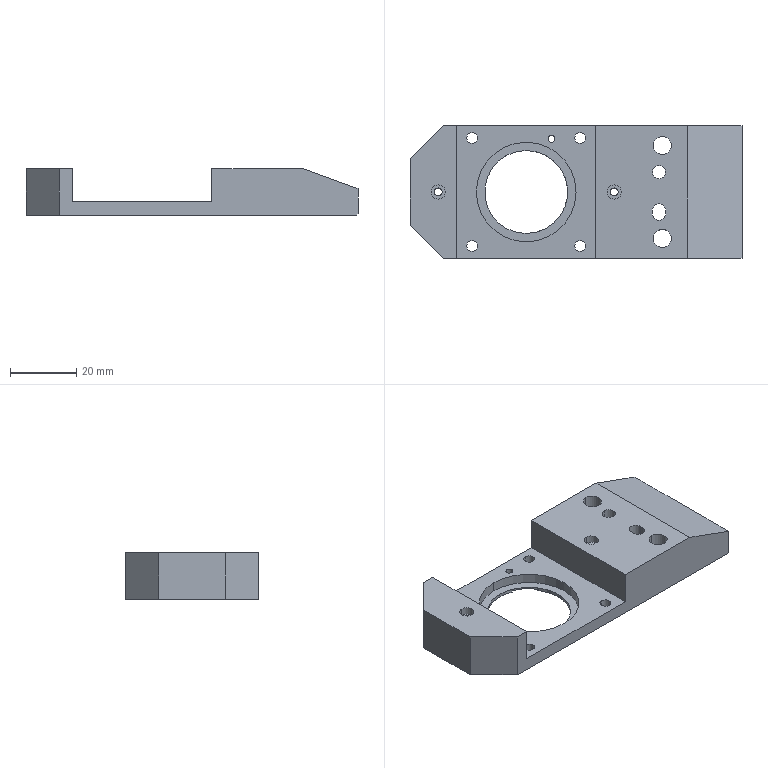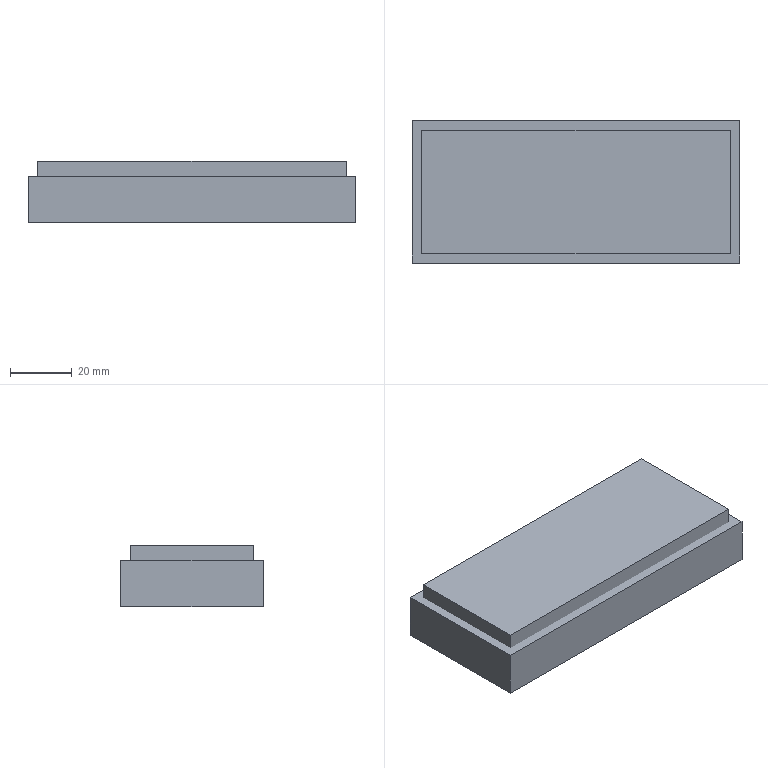CAM job | NX | 3-axis milling, drilling | part box 100 x 40 x 14 mm | stock box 106 x 46 x 20 mm
Tools:
number,name,description,diameter,corner_radius,flute_length,length,flutes
3,D50R0.8,Milling Tool-5 Parameters,50.0,0.8,50.0,75.0,2
4,D10,Milling Tool-5 Parameters,10.0,0.0,50.0,75.0,2
20,ZXZ,Milling Tool-5 Parameters,6.0,0.0,50.0,75.0,2
13,3.3ZT,Drilling Tool,3.3,0.0,35.0,50.0,2
11,D2.9XYD,Thread Mill,2.9,0.0,0.7,50.0,2
9,3.8ZT,Drilling Tool,3.8,0.0,35.0,50.0,2
10,4.0JD,Milling Tool-5 Parameters,4.0,0.0,30.0,30.0,4
12,5.5ZT,Drilling Tool,5.5,0.0,35.0,50.0,2
19,2.4ZT,Drilling Tool,2.4,0.0,35.0,50.0,2
15,2.1ZT,Drilling Tool,2.05,0.0,35.0,50.0,2
7,1.95XYD,Thread Mill,1.95,0.0,0.45,50.0,2
16,D6JING,Milling Tool-5 Parameters,6.0,0.0,50.0,75.0,2
14,D10JING,Milling Tool-5 Parameters,10.0,0.0,50.0,75.0,2
8,D6R0.5,Milling Tool-5 Parameters,6.0,0.5,50.0,75.0,2
17,D3,Milling Tool-5 Parameters,3.0,0.0,50.0,75.0,2
1,D6A45,Milling Tool-5 Parameters,6.0,0.0,3.0,3.0,2
6,D6,Milling Tool-5 Parameters,6.0,0.0,50.0,75.0,2
Operations:
program,operation,operation_type,tool,method,geometry_group,spindle_rpm,surface_speed,feed_per_tooth,feed_cut,feed_plunge,cut_length_mm,path_length_mm,cut_time_min,machine_time_min
1,FLOOR_WALL_COPY,VolumeBased25DMillingOperation,D50R0.8,METHOD,A,1500.0,296.0,0.3333,1000.0,100.0,168.0,222.0,0.168,0.1734
1,ADAPTIVE_MILLING_COPY,CavityMilling,D10,METHOD,A,4000.0,125.0,0.275,2200.0,1000.0,26621.985,27666.782,13.445,13.55
1,ZLEVEL_PROFILE_1_COPY_1,ZLevelMilling,D10,METHOD,A,3500.0,109.0,0.2857,2000.0,100.0,150.755,235.284,0.0754,0.0838
1,DRILLING_COPY_1,Operation,ZXZ,METHOD,A,5000.0,94.0,0.025,250.0,0.0,48.0,392.654,0.192,0.2265
1,DRILLING_COPY_1_COPY,Operation,3.3ZT,METHOD,A,2000.0,21.0,0.0375,150.0,0.0,33.966,254.926,0.2264,0.2485
1,TOOLCOMP11,ThreadMilling,D2.9XYD,METHOD,A,4000.0,36.0,0.125,1000.0,100.0,301.86,1748.914,0.3019,0.4466
1,DRILLING_COPY_1_COPY_COPY_2,Operation,2.1ZT,METHOD,A,2001.0,12.0,0.03,120.0,0.0,7.616,95.232,0.0635,0.0722
1,TOOLCOMP7,ThreadMilling,1.95XYD,METHOD,A,4000.0,36.0,0.125,1000.0,100.0,37.492,286.492,0.0375,0.0624
1,DRILLING_COPY_2,HoleDrilling,3.8ZT,METHOD,A,2000.0,23.0,0.0375,150.0,0.0,381.687,425.187,0.2456,0.25
1,DRILLING_COPY_2_COPY,HoleDrilling,4.0JD,METHOD,A,1000.0,12.0,0.0125,50.0,0.0,35.0,51.0,0.35,0.3516
1,DRILLING_COPY_1_COPY_COPY,Operation,5.5ZT,METHOD,A,1215.0,21.0,0.0617,150.0,0.0,37.305,165.77,0.2487,0.2615
1,DRILLING_COPY_1_COPY_COPY_1,Operation,2.4ZT,METHOD,A,2785.0,21.0,0.018,100.0,0.0,35.442,186.969,0.3544,0.3696
1,ZLEVEL_PROFILE_1_COPY,ZLevelMilling,D10JING,METHOD,A,6500.0,122.0,0.0769,1000.0,100.0,357.473,643.22,0.3575,0.386
1,FLOOR_WALL,VolumeBased25DMillingOperation,D10JING,METHOD,A,6500.0,122.0,0.0962,1250.0,100.0,546.488,811.524,0.4372,0.4637
1,ZLEVEL_PROFILE_COPY_COPY_COPY_COPY,ZLevelMilling,D6R0.5,METHOD,A,6500.0,122.0,0.1923,2500.0,1000.0,8190.857,8255.391,3.278,3.284
1,HOLE_MILLING,CylinderMilling,D3,METHOD,A,5500.0,51.0,0.1136,1250.0,100.0,393.473,570.073,0.3148,0.3324
1,ZLEVEL_PROFILE_COPY_COPY_COPY,ZLevelMilling,D3,METHOD,A,4500.0,42.0,0.1333,1200.0,1000.0,1148.263,1220.263,0.9603,0.9675
1,11_COPY_COPY_COPY_COPY,ZLevelMilling,D6A45,METHOD,A,7500.0,141.0,0.0667,1000.0,100.0,319.125,1014.636,0.3191,0.3887
1,11_COPY_COPY_COPY_COPY_COPY,ZLevelMilling,D6A45,METHOD,A,7500.0,141.0,0.0667,1000.0,100.0,235.065,969.548,0.2351,0.3085
1,TOOLCOMP14,VolumeBased25DMillingOperation,D10JING,METHOD,A,9500.0,179.0,0.0658,1250.0,100.0,68.154,152.154,0.0545,0.0629
1,TOOLCOMP17,VolumeBased25DMillingOperation,D3,METHOD,A,6000.0,56.0,0.0667,800.0,100.0,79.224,151.224,0.099,0.1062
2,FLOOR_WALL_COPY_COPY,VolumeBased25DMillingOperation,D50R0.8,METHOD,B,1000.0,157.0,0.75,1500.0,100.0,3240.0,7166.852,2.16,2.553
2,FLOOR_WALL_COPY_COPY_1,VolumeBased25DMillingOperation,D50R0.8,METHOD,B,1500.0,296.0,0.3333,1000.0,100.0,162.0,216.0,0.162,0.1674
2,HOLE_MILLING_1,CylinderMilling,D6,METHOD,B,4000.0,75.0,0.225,1800.0,100.0,1932.36,2294.916,1.073,1.11
2,HOLE_MILLING_1_COPY,CylinderMilling,D6JING,METHOD,B,5500.0,103.0,0.0909,1000.0,100.0,150.223,512.779,0.1502,0.1865
2,FLOOR_WALL_COPY_1,VolumeBased25DMillingOperation,D6JING,METHOD,B,6500.0,122.0,0.0962,1250.0,100.0,159.806,395.144,0.1278,0.1514
2,HOLE_MILLING_COPY,CylinderMilling,D3,METHOD,B,5500.0,51.0,0.1136,1250.0,100.0,272.435,473.036,0.2179,0.238
2,11_COPY_COPY_COPY_COPY_COPY_1,ZLevelMilling,D6A45,METHOD,B,7500.0,141.0,0.0667,1000.0,100.0,575.293,1745.696,0.5753,0.6923
2,TOOLCOMP17.,CylinderMilling,D3,METHOD,B,6500.0,61.0,0.0654,850.0,100.0,25.77,226.37,0.0303,0.0504